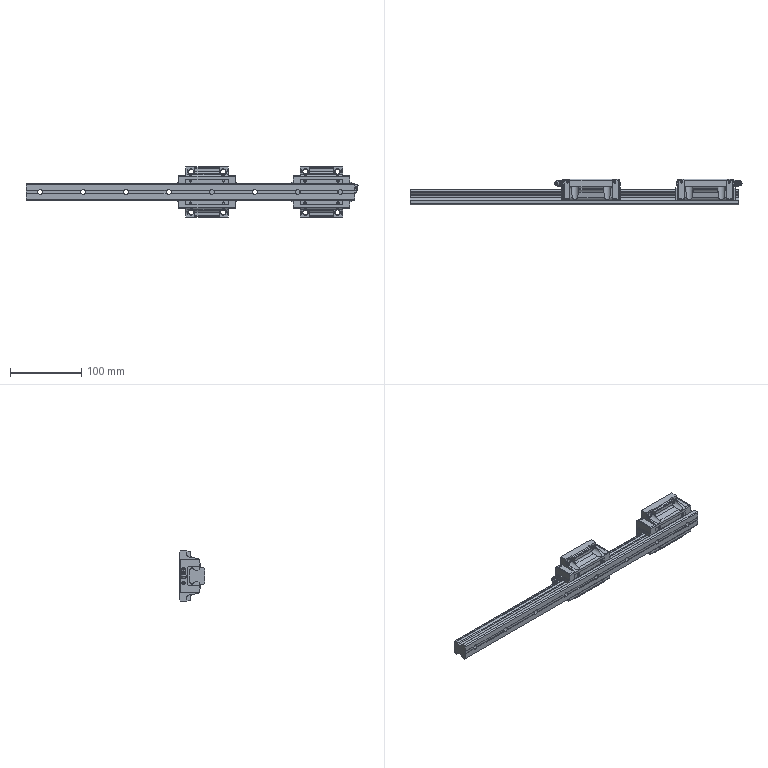Part | SolidWorks | 5 solids | 762 faces | box 464.6 x 36 x 70 mm | volume 394256 mm3 | plane 442 | cylinder 192 | cone 72 | torus 44 | sphere 12 | commonest cylinder face diameters 11 x28 10 x24 3 x16 3.518 x16 4.5 x16 4.917 x16